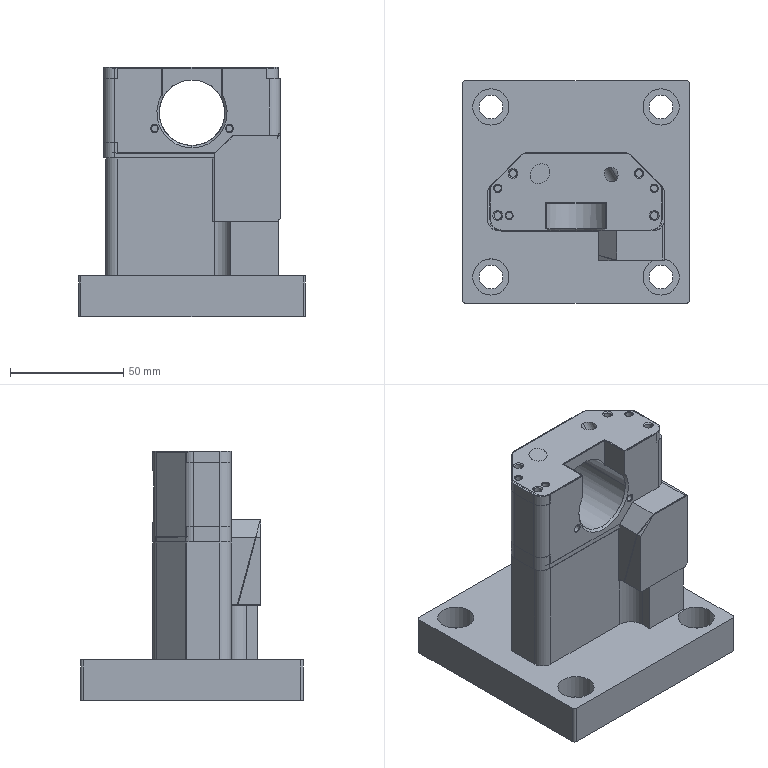Part | 3 solids | 388 faces | box 100 x 98 x 110 mm | volume 437079 mm3 | plane 169 | cylinder 122 | cone 94 | sphere 3 | commonest cylinder face diameters 10 x21 3 x20 3.3 x20 4.2 x8 6 x8 20 x8